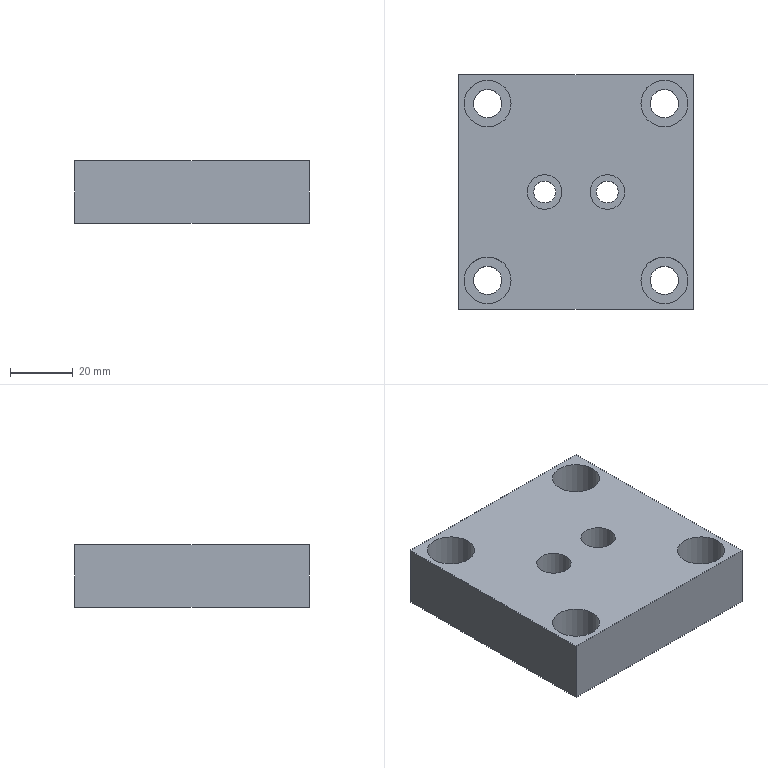Part | NX | features solid 2 | 1 solid | 24 faces | box 75 x 75 x 20 mm | volume 99312 mm3 | plane 12 | cylinder 12 | commonest cylinder face diameters 9 x4 15 x4 7 x2 11 x2
STEP:
#1=CARTESIAN_POINT('',(-127.5,292.5,330.));
#2=VERTEX_POINT('',#1);
#3=CARTESIAN_POINT('',(-127.5,292.5,350.));
#4=VERTEX_POINT('',#3);
#5=CARTESIAN_POINT('',(-127.5,292.5,350.));
#6=DIRECTION('',(0.,0.,-1.));
#7=VECTOR('',#6,1000.);
#8=LINE('',#5,#7);
#9=EDGE_CURVE('',#2,#4,#8,.F.);
#10=ORIENTED_EDGE('',*,*,#9,.T.);
#11=CARTESIAN_POINT('',(-52.5,292.5,350.));
#12=VERTEX_POINT('',#11);
#13=CARTESIAN_POINT('',(-205.,292.5,350.));
#14=DIRECTION('',(1.,0.,0.));
#15=VECTOR('',#14,1000.);
#16=LINE('',#13,#15);
#17=EDGE_CURVE('',#12,#4,#16,.F.);
#18=ORIENTED_EDGE('',*,*,#17,.F.);
#19=CARTESIAN_POINT('',(-52.5,292.5,330.));
#20=VERTEX_POINT('',#19);
#21=CARTESIAN_POINT('',(-52.5,292.5,350.));
#22=DIRECTION('',(0.,0.,1.));
#23=VECTOR('',#22,1000.);
#24=LINE('',#21,#23);
#25=EDGE_CURVE('',#20,#12,#24,.T.);
#26=ORIENTED_EDGE('',*,*,#25,.F.);
#27=CARTESIAN_POINT('',(-92.5,292.5,330.));
#28=DIRECTION('',(-1.,0.,0.));
#29=VECTOR('',#28,1000.);
#30=LINE('',#27,#29);
#31=EDGE_CURVE('',#20,#2,#30,.T.);
#32=ORIENTED_EDGE('',*,*,#31,.T.);
#33=EDGE_LOOP('',(#10,#18,#26,#32));
#34=FACE_BOUND('',#33,.T.);
#35=CARTESIAN_POINT('',(-62.5,292.5,350.));
#36=DIRECTION('',(0.,1.,0.));
#37=DIRECTION('',(-1.,0.,0.));
#38=AXIS2_PLACEMENT_3D('',#35,#36,#37);
#39=PLANE('',#38);
#40=ADVANCED_FACE('',(#34),#39,.T.);
#41=ORIENTED_EDGE('',*,*,#25,.T.);
#42=CARTESIAN_POINT('',(-52.5,217.5,350.));
#43=VERTEX_POINT('',#42);
#44=CARTESIAN_POINT('',(-52.5,50.,350.));
#45=DIRECTION('',(0.,-1.,0.));
#46=VECTOR('',#45,1000.);
#47=LINE('',#44,#46);
#48=EDGE_CURVE('',#43,#12,#47,.F.);
#49=ORIENTED_EDGE('',*,*,#48,.F.);
#50=CARTESIAN_POINT('',(-52.5,217.5,330.));
#51=VERTEX_POINT('',#50);
#52=CARTESIAN_POINT('',(-52.5,217.5,350.));
#53=DIRECTION('',(0.,0.,-1.));
#54=VECTOR('',#53,1000.);
#55=LINE('',#52,#54);
#56=EDGE_CURVE('',#51,#43,#55,.F.);
#57=ORIENTED_EDGE('',*,*,#56,.F.);
#58=CARTESIAN_POINT('',(-52.5,222.5,330.));
#59=DIRECTION('',(0.,1.,0.));
#60=VECTOR('',#59,1000.);
#61=LINE('',#58,#60);
#62=EDGE_CURVE('',#51,#20,#61,.T.);
#63=ORIENTED_EDGE('',*,*,#62,.T.);
#64=EDGE_LOOP('',(#41,#49,#57,#63));
#65=FACE_BOUND('',#64,.T.);
#66=CARTESIAN_POINT('',(-52.5,227.5,350.));
#67=DIRECTION('',(1.,0.,0.));
#68=DIRECTION('',(0.,0.,-1.));
#69=AXIS2_PLACEMENT_3D('',#66,#67,#68);
#70=PLANE('',#69);
#71=ADVANCED_FACE('',(#65),#70,.T.);
#72=ORIENTED_EDGE('',*,*,#56,.T.);
#73=CARTESIAN_POINT('',(-127.5,217.5,350.));
#74=VERTEX_POINT('',#73);
#75=CARTESIAN_POINT('',(-205.,217.5,350.));
#76=DIRECTION('',(-1.,0.,0.));
#77=VECTOR('',#76,1000.);
#78=LINE('',#75,#77);
#79=EDGE_CURVE('',#43,#74,#78,.T.);
#80=ORIENTED_EDGE('',*,*,#79,.T.);
#81=CARTESIAN_POINT('',(-127.5,217.5,330.));
#82=VERTEX_POINT('',#81);
#83=CARTESIAN_POINT('',(-127.5,217.5,350.));
#84=DIRECTION('',(0.,0.,1.));
#85=VECTOR('',#84,1000.);
#86=LINE('',#83,#85);
#87=EDGE_CURVE('',#82,#74,#86,.T.);
#88=ORIENTED_EDGE('',*,*,#87,.F.);
#89=CARTESIAN_POINT('',(-92.5,217.5,330.));
#90=DIRECTION('',(1.,0.,0.));
#91=VECTOR('',#90,1000.);
#92=LINE('',#89,#91);
#93=EDGE_CURVE('',#51,#82,#92,.F.);
#94=ORIENTED_EDGE('',*,*,#93,.F.);
#95=EDGE_LOOP('',(#72,#80,#88,#94));
#96=FACE_BOUND('',#95,.T.);
#97=CARTESIAN_POINT('',(-117.5,217.5,350.));
#98=DIRECTION('',(0.,-1.,0.));
#99=DIRECTION('',(0.,0.,-1.));
#100=AXIS2_PLACEMENT_3D('',#97,#98,#99);
#101=PLANE('',#100);
#102=ADVANCED_FACE('',(#96),#101,.T.);
#103=CARTESIAN_POINT('',(-127.5,50.,350.));
#104=DIRECTION('',(0.,1.,0.));
#105=VECTOR('',#104,1000.);
#106=LINE('',#103,#105);
#107=EDGE_CURVE('',#74,#4,#106,.T.);
#108=ORIENTED_EDGE('',*,*,#107,.T.);
#109=ORIENTED_EDGE('',*,*,#9,.F.);
#110=CARTESIAN_POINT('',(-127.5,222.5,330.));
#111=DIRECTION('',(0.,-1.,0.));
#112=VECTOR('',#111,1000.);
#113=LINE('',#110,#112);
#114=EDGE_CURVE('',#82,#2,#113,.F.);
#115=ORIENTED_EDGE('',*,*,#114,.F.);
#116=ORIENTED_EDGE('',*,*,#87,.T.);
#117=EDGE_LOOP('',(#108,#109,#115,#116));
#118=FACE_BOUND('',#117,.T.);
#119=CARTESIAN_POINT('',(-127.5,252.5,350.));
#120=DIRECTION('',(-1.,0.,0.));
#121=DIRECTION('',(0.,1.,0.));
#122=AXIS2_PLACEMENT_3D('',#119,#120,#121);
#123=PLANE('',#122);
#124=ADVANCED_FACE('',(#118),#123,.T.);
#125=CARTESIAN_POINT('',(-83.5,255.,330.));
#126=VERTEX_POINT('',#125);
#127=CARTESIAN_POINT('',(-80.,255.,330.));
#128=DIRECTION('',(0.,0.,-1.));
#129=DIRECTION('',(-1.,0.,0.));
#130=AXIS2_PLACEMENT_3D('',#127,#128,#129);
#131=CIRCLE('',#130,3.5);
#132=EDGE_CURVE('',#126,#126,#131,.T.);
#133=ORIENTED_EDGE('',*,*,#132,.F.);
#134=EDGE_LOOP('',(#133));
#135=FACE_BOUND('',#134,.T.);
#136=CARTESIAN_POINT('',(-103.5,255.,330.));
#137=VERTEX_POINT('',#136);
#138=CARTESIAN_POINT('',(-100.,255.,330.));
#139=DIRECTION('',(0.,0.,-1.));
#140=DIRECTION('',(-1.,0.,0.));
#141=AXIS2_PLACEMENT_3D('',#138,#139,#140);
#142=CIRCLE('',#141,3.5);
#143=EDGE_CURVE('',#137,#137,#142,.T.);
#144=ORIENTED_EDGE('',*,*,#143,.F.);
#145=EDGE_LOOP('',(#144));
#146=FACE_BOUND('',#145,.T.);
#147=CARTESIAN_POINT('',(-66.25,226.75,330.));
#148=VERTEX_POINT('',#147);
#149=CARTESIAN_POINT('',(-61.75,226.75,330.));
#150=DIRECTION('',(0.,0.,-1.));
#151=DIRECTION('',(-1.,0.,0.));
#152=AXIS2_PLACEMENT_3D('',#149,#150,#151);
#153=CIRCLE('',#152,4.5);
#154=EDGE_CURVE('',#148,#148,#153,.T.);
#155=ORIENTED_EDGE('',*,*,#154,.F.);
#156=EDGE_LOOP('',(#155));
#157=FACE_BOUND('',#156,.T.);
#158=CARTESIAN_POINT('',(-122.75,226.75,330.));
#159=VERTEX_POINT('',#158);
#160=CARTESIAN_POINT('',(-118.25,226.75,330.));
#161=DIRECTION('',(0.,0.,-1.));
#162=DIRECTION('',(-1.,0.,0.));
#163=AXIS2_PLACEMENT_3D('',#160,#161,#162);
#164=CIRCLE('',#163,4.5);
#165=EDGE_CURVE('',#159,#159,#164,.T.);
#166=ORIENTED_EDGE('',*,*,#165,.F.);
#167=EDGE_LOOP('',(#166));
#168=FACE_BOUND('',#167,.T.);
#169=CARTESIAN_POINT('',(-66.25,283.25,330.));
#170=VERTEX_POINT('',#169);
#171=CARTESIAN_POINT('',(-61.75,283.25,330.));
#172=DIRECTION('',(0.,0.,-1.));
#173=DIRECTION('',(-1.,0.,0.));
#174=AXIS2_PLACEMENT_3D('',#171,#172,#173);
#175=CIRCLE('',#174,4.5);
#176=EDGE_CURVE('',#170,#170,#175,.T.);
#177=ORIENTED_EDGE('',*,*,#176,.F.);
#178=EDGE_LOOP('',(#177));
#179=FACE_BOUND('',#178,.T.);
#180=CARTESIAN_POINT('',(-122.75,283.25,330.));
#181=VERTEX_POINT('',#180);
#182=CARTESIAN_POINT('',(-118.25,283.25,330.));
#183=DIRECTION('',(0.,0.,-1.));
#184=DIRECTION('',(-1.,0.,0.));
#185=AXIS2_PLACEMENT_3D('',#182,#183,#184);
#186=CIRCLE('',#185,4.5);
#187=EDGE_CURVE('',#181,#181,#186,.T.);
#188=ORIENTED_EDGE('',*,*,#187,.F.);
#189=EDGE_LOOP('',(#188));
#190=FACE_BOUND('',#189,.T.);
#191=ORIENTED_EDGE('',*,*,#31,.F.);
#192=ORIENTED_EDGE('',*,*,#62,.F.);
#193=ORIENTED_EDGE('',*,*,#93,.T.);
#194=ORIENTED_EDGE('',*,*,#114,.T.);
#195=EDGE_LOOP('',(#191,#192,#193,#194));
#196=FACE_BOUND('',#195,.T.);
#197=CARTESIAN_POINT('',(-92.5,222.5,330.));
#198=DIRECTION('',(0.,0.,-1.));
#199=DIRECTION('',(0.,1.,0.));
#200=AXIS2_PLACEMENT_3D('',#197,#198,#199);
#201=PLANE('',#200);
#202=ADVANCED_FACE('',(#135,#146,#157,#168,#179,#190,#196),#201,.T.);
#203=CARTESIAN_POINT('',(-85.5,255.,350.));
#204=VERTEX_POINT('',#203);
#205=CARTESIAN_POINT('',(-80.,255.,350.));
#206=DIRECTION('',(0.,0.,-1.));
#207=DIRECTION('',(-1.,0.,0.));
#208=AXIS2_PLACEMENT_3D('',#205,#206,#207);
#209=CIRCLE('',#208,5.5);
#210=EDGE_CURVE('',#204,#204,#209,.T.);
#211=ORIENTED_EDGE('',*,*,#210,.T.);
#212=EDGE_LOOP('',(#211));
#213=FACE_BOUND('',#212,.T.);
#214=CARTESIAN_POINT('',(-105.5,255.,350.));
#215=VERTEX_POINT('',#214);
#216=CARTESIAN_POINT('',(-100.,255.,350.));
#217=DIRECTION('',(0.,0.,-1.));
#218=DIRECTION('',(-1.,0.,0.));
#219=AXIS2_PLACEMENT_3D('',#216,#217,#218);
#220=CIRCLE('',#219,5.5);
#221=EDGE_CURVE('',#215,#215,#220,.T.);
#222=ORIENTED_EDGE('',*,*,#221,.T.);
#223=EDGE_LOOP('',(#222));
#224=FACE_BOUND('',#223,.T.);
#225=CARTESIAN_POINT('',(-69.25,226.75,350.));
#226=VERTEX_POINT('',#225);
#227=CARTESIAN_POINT('',(-61.75,226.75,350.));
#228=DIRECTION('',(0.,0.,-1.));
#229=DIRECTION('',(-1.,0.,0.));
#230=AXIS2_PLACEMENT_3D('',#227,#228,#229);
#231=CIRCLE('',#230,7.5);
#232=EDGE_CURVE('',#226,#226,#231,.T.);
#233=ORIENTED_EDGE('',*,*,#232,.T.);
#234=EDGE_LOOP('',(#233));
#235=FACE_BOUND('',#234,.T.);
#236=CARTESIAN_POINT('',(-125.75,226.75,350.));
#237=VERTEX_POINT('',#236);
#238=CARTESIAN_POINT('',(-118.25,226.75,350.));
#239=DIRECTION('',(0.,0.,-1.));
#240=DIRECTION('',(-1.,0.,0.));
#241=AXIS2_PLACEMENT_3D('',#238,#239,#240);
#242=CIRCLE('',#241,7.5);
#243=EDGE_CURVE('',#237,#237,#242,.T.);
#244=ORIENTED_EDGE('',*,*,#243,.T.);
#245=EDGE_LOOP('',(#244));
#246=FACE_BOUND('',#245,.T.);
#247=CARTESIAN_POINT('',(-69.25,283.25,350.));
#248=VERTEX_POINT('',#247);
#249=CARTESIAN_POINT('',(-61.75,283.25,350.));
#250=DIRECTION('',(0.,0.,-1.));
#251=DIRECTION('',(-1.,0.,0.));
#252=AXIS2_PLACEMENT_3D('',#249,#250,#251);
#253=CIRCLE('',#252,7.5);
#254=EDGE_CURVE('',#248,#248,#253,.T.);
#255=ORIENTED_EDGE('',*,*,#254,.T.);
#256=EDGE_LOOP('',(#255));
#257=FACE_BOUND('',#256,.T.);
#258=CARTESIAN_POINT('',(-125.75,283.25,350.));
#259=VERTEX_POINT('',#258);
#260=CARTESIAN_POINT('',(-118.25,283.25,350.));
#261=DIRECTION('',(0.,0.,-1.));
#262=DIRECTION('',(-1.,0.,0.));
#263=AXIS2_PLACEMENT_3D('',#260,#261,#262);
#264=CIRCLE('',#263,7.5);
#265=EDGE_CURVE('',#259,#259,#264,.T.);
#266=ORIENTED_EDGE('',*,*,#265,.T.);
#267=EDGE_LOOP('',(#266));
#268=FACE_BOUND('',#267,.T.);
#269=ORIENTED_EDGE('',*,*,#48,.T.);
#270=ORIENTED_EDGE('',*,*,#17,.T.);
#271=ORIENTED_EDGE('',*,*,#107,.F.);
#272=ORIENTED_EDGE('',*,*,#79,.F.);
#273=EDGE_LOOP('',(#269,#270,#271,#272));
#274=FACE_BOUND('',#273,.T.);
#275=CARTESIAN_POINT('',(-205.,50.,350.));
#276=DIRECTION('',(0.,0.,1.));
#277=DIRECTION('',(1.,0.,0.));
#278=AXIS2_PLACEMENT_3D('',#275,#276,#277);
#279=PLANE('',#278);
#280=ADVANCED_FACE('',(#213,#224,#235,#246,#257,#268,#274),#279,.T.);
#281=ORIENTED_EDGE('',*,*,#187,.T.);
#282=EDGE_LOOP('',(#281));
#283=FACE_BOUND('',#282,.T.);
#284=CARTESIAN_POINT('',(-122.75,283.25,338.));
#285=VERTEX_POINT('',#284);
#286=CARTESIAN_POINT('',(-118.25,283.25,338.));
#287=DIRECTION('',(0.,0.,-1.));
#288=DIRECTION('',(-1.,0.,0.));
#289=AXIS2_PLACEMENT_3D('',#286,#287,#288);
#290=CIRCLE('',#289,4.5);
#291=EDGE_CURVE('',#285,#285,#290,.T.);
#292=ORIENTED_EDGE('',*,*,#291,.F.);
#293=EDGE_LOOP('',(#292));
#294=FACE_BOUND('',#293,.T.);
#295=CARTESIAN_POINT('',(-118.25,283.25,300.));
#296=DIRECTION('',(0.,0.,-1.));
#297=DIRECTION('',(-1.,0.,0.));
#298=AXIS2_PLACEMENT_3D('',#295,#296,#297);
#299=CYLINDRICAL_SURFACE('',#298,4.5);
#300=ADVANCED_FACE('',(#283,#294),#299,.F.);
#301=ORIENTED_EDGE('',*,*,#291,.T.);
#302=EDGE_LOOP('',(#301));
#303=FACE_BOUND('',#302,.T.);
#304=CARTESIAN_POINT('',(-125.75,283.25,338.));
#305=VERTEX_POINT('',#304);
#306=CARTESIAN_POINT('',(-118.25,283.25,338.));
#307=DIRECTION('',(0.,0.,-1.));
#308=DIRECTION('',(-1.,0.,0.));
#309=AXIS2_PLACEMENT_3D('',#306,#307,#308);
#310=CIRCLE('',#309,7.5);
#311=EDGE_CURVE('',#305,#305,#310,.T.);
#312=ORIENTED_EDGE('',*,*,#311,.F.);
#313=EDGE_LOOP('',(#312));
#314=FACE_BOUND('',#313,.T.);
#315=CARTESIAN_POINT('',(-107.5,272.5,338.));
#316=DIRECTION('',(0.,0.,-1.));
#317=DIRECTION('',(-1.,0.,0.));
#318=AXIS2_PLACEMENT_3D('',#315,#316,#317);
#319=PLANE('',#318);
#320=ADVANCED_FACE('',(#303,#314),#319,.F.);
#321=ORIENTED_EDGE('',*,*,#311,.T.);
#322=EDGE_LOOP('',(#321));
#323=FACE_BOUND('',#322,.T.);
#324=ORIENTED_EDGE('',*,*,#265,.F.);
#325=EDGE_LOOP('',(#324));
#326=FACE_BOUND('',#325,.T.);
#327=CARTESIAN_POINT('',(-118.25,283.25,350.));
#328=DIRECTION('',(0.,0.,-1.));
#329=DIRECTION('',(-1.,0.,0.));
#330=AXIS2_PLACEMENT_3D('',#327,#328,#329);
#331=CYLINDRICAL_SURFACE('',#330,7.5);
#332=ADVANCED_FACE('',(#323,#326),#331,.F.);
#333=ORIENTED_EDGE('',*,*,#176,.T.);
#334=EDGE_LOOP('',(#333));
#335=FACE_BOUND('',#334,.T.);
#336=CARTESIAN_POINT('',(-66.25,283.25,338.));
#337=VERTEX_POINT('',#336);
#338=CARTESIAN_POINT('',(-61.75,283.25,338.));
#339=DIRECTION('',(0.,0.,-1.));
#340=DIRECTION('',(-1.,0.,0.));
#341=AXIS2_PLACEMENT_3D('',#338,#339,#340);
#342=CIRCLE('',#341,4.5);
#343=EDGE_CURVE('',#337,#337,#342,.T.);
#344=ORIENTED_EDGE('',*,*,#343,.F.);
#345=EDGE_LOOP('',(#344));
#346=FACE_BOUND('',#345,.T.);
#347=CARTESIAN_POINT('',(-61.75,283.25,300.));
#348=DIRECTION('',(0.,0.,-1.));
#349=DIRECTION('',(-1.,0.,0.));
#350=AXIS2_PLACEMENT_3D('',#347,#348,#349);
#351=CYLINDRICAL_SURFACE('',#350,4.5);
#352=ADVANCED_FACE('',(#335,#346),#351,.F.);
#353=ORIENTED_EDGE('',*,*,#343,.T.);
#354=EDGE_LOOP('',(#353));
#355=FACE_BOUND('',#354,.T.);
#356=CARTESIAN_POINT('',(-69.25,283.25,338.));
#357=VERTEX_POINT('',#356);
#358=CARTESIAN_POINT('',(-61.75,283.25,338.));
#359=DIRECTION('',(0.,0.,-1.));
#360=DIRECTION('',(-1.,0.,0.));
#361=AXIS2_PLACEMENT_3D('',#358,#359,#360);
#362=CIRCLE('',#361,7.5);
#363=EDGE_CURVE('',#357,#357,#362,.T.);
#364=ORIENTED_EDGE('',*,*,#363,.F.);
#365=EDGE_LOOP('',(#364));
#366=FACE_BOUND('',#365,.T.);
#367=CARTESIAN_POINT('',(-72.5,272.5,338.));
#368=DIRECTION('',(0.,0.,-1.));
#369=DIRECTION('',(-1.,0.,0.));
#370=AXIS2_PLACEMENT_3D('',#367,#368,#369);
#371=PLANE('',#370);
#372=ADVANCED_FACE('',(#355,#366),#371,.F.);
#373=ORIENTED_EDGE('',*,*,#363,.T.);
#374=EDGE_LOOP('',(#373));
#375=FACE_BOUND('',#374,.T.);
#376=ORIENTED_EDGE('',*,*,#254,.F.);
#377=EDGE_LOOP('',(#376));
#378=FACE_BOUND('',#377,.T.);
#379=CARTESIAN_POINT('',(-61.75,283.25,350.));
#380=DIRECTION('',(0.,0.,-1.));
#381=DIRECTION('',(-1.,0.,0.));
#382=AXIS2_PLACEMENT_3D('',#379,#380,#381);
#383=CYLINDRICAL_SURFACE('',#382,7.5);
#384=ADVANCED_FACE('',(#375,#378),#383,.F.);
#385=ORIENTED_EDGE('',*,*,#165,.T.);
#386=EDGE_LOOP('',(#385));
#387=FACE_BOUND('',#386,.T.);
#388=CARTESIAN_POINT('',(-122.75,226.75,338.));
#389=VERTEX_POINT('',#388);
#390=CARTESIAN_POINT('',(-118.25,226.75,338.));
#391=DIRECTION('',(0.,0.,-1.));
#392=DIRECTION('',(-1.,0.,0.));
#393=AXIS2_PLACEMENT_3D('',#390,#391,#392);
#394=CIRCLE('',#393,4.5);
#395=EDGE_CURVE('',#389,#389,#394,.T.);
#396=ORIENTED_EDGE('',*,*,#395,.F.);
#397=EDGE_LOOP('',(#396));
#398=FACE_BOUND('',#397,.T.);
#399=CARTESIAN_POINT('',(-118.25,226.75,300.));
#400=DIRECTION('',(0.,0.,-1.));
#401=DIRECTION('',(-1.,0.,0.));
#402=AXIS2_PLACEMENT_3D('',#399,#400,#401);
#403=CYLINDRICAL_SURFACE('',#402,4.5);
#404=ADVANCED_FACE('',(#387,#398),#403,.F.);
#405=ORIENTED_EDGE('',*,*,#395,.T.);
#406=EDGE_LOOP('',(#405));
#407=FACE_BOUND('',#406,.T.);
#408=CARTESIAN_POINT('',(-125.75,226.75,338.));
#409=VERTEX_POINT('',#408);
#410=CARTESIAN_POINT('',(-118.25,226.75,338.));
#411=DIRECTION('',(0.,0.,-1.));
#412=DIRECTION('',(-1.,0.,0.));
#413=AXIS2_PLACEMENT_3D('',#410,#411,#412);
#414=CIRCLE('',#413,7.5);
#415=EDGE_CURVE('',#409,#409,#414,.T.);
#416=ORIENTED_EDGE('',*,*,#415,.F.);
#417=EDGE_LOOP('',(#416));
#418=FACE_BOUND('',#417,.T.);
#419=CARTESIAN_POINT('',(-107.5,237.5,338.));
#420=DIRECTION('',(0.,0.,-1.));
#421=DIRECTION('',(-1.,0.,0.));
#422=AXIS2_PLACEMENT_3D('',#419,#420,#421);
#423=PLANE('',#422);
#424=ADVANCED_FACE('',(#407,#418),#423,.F.);
#425=ORIENTED_EDGE('',*,*,#415,.T.);
#426=EDGE_LOOP('',(#425));
#427=FACE_BOUND('',#426,.T.);
#428=ORIENTED_EDGE('',*,*,#243,.F.);
#429=EDGE_LOOP('',(#428));
#430=FACE_BOUND('',#429,.T.);
#431=CARTESIAN_POINT('',(-118.25,226.75,350.));
#432=DIRECTION('',(0.,0.,-1.));
#433=DIRECTION('',(-1.,0.,0.));
#434=AXIS2_PLACEMENT_3D('',#431,#432,#433);
#435=CYLINDRICAL_SURFACE('',#434,7.5);
#436=ADVANCED_FACE('',(#427,#430),#435,.F.);
#437=ORIENTED_EDGE('',*,*,#154,.T.);
#438=EDGE_LOOP('',(#437));
#439=FACE_BOUND('',#438,.T.);
#440=CARTESIAN_POINT('',(-66.25,226.75,338.));
#441=VERTEX_POINT('',#440);
#442=CARTESIAN_POINT('',(-61.75,226.75,338.));
#443=DIRECTION('',(0.,0.,-1.));
#444=DIRECTION('',(-1.,0.,0.));
#445=AXIS2_PLACEMENT_3D('',#442,#443,#444);
#446=CIRCLE('',#445,4.5);
#447=EDGE_CURVE('',#441,#441,#446,.T.);
#448=ORIENTED_EDGE('',*,*,#447,.F.);
#449=EDGE_LOOP('',(#448));
#450=FACE_BOUND('',#449,.T.);
#451=CARTESIAN_POINT('',(-61.75,226.75,300.));
#452=DIRECTION('',(0.,0.,-1.));
#453=DIRECTION('',(-1.,0.,0.));
#454=AXIS2_PLACEMENT_3D('',#451,#452,#453);
#455=CYLINDRICAL_SURFACE('',#454,4.5);
#456=ADVANCED_FACE('',(#439,#450),#455,.F.);
#457=ORIENTED_EDGE('',*,*,#447,.T.);
#458=EDGE_LOOP('',(#457));
#459=FACE_BOUND('',#458,.T.);
#460=CARTESIAN_POINT('',(-69.25,226.75,338.));
#461=VERTEX_POINT('',#460);
#462=CARTESIAN_POINT('',(-61.75,226.75,338.));
#463=DIRECTION('',(0.,0.,-1.));
#464=DIRECTION('',(-1.,0.,0.));
#465=AXIS2_PLACEMENT_3D('',#462,#463,#464);
#466=CIRCLE('',#465,7.5);
#467=EDGE_CURVE('',#461,#461,#466,.T.);
#468=ORIENTED_EDGE('',*,*,#467,.F.);
#469=EDGE_LOOP('',(#468));
#470=FACE_BOUND('',#469,.T.);
#471=CARTESIAN_POINT('',(-72.5,237.5,338.));
#472=DIRECTION('',(0.,0.,-1.));
#473=DIRECTION('',(-1.,0.,0.));
#474=AXIS2_PLACEMENT_3D('',#471,#472,#473);
#475=PLANE('',#474);
#476=ADVANCED_FACE('',(#459,#470),#475,.F.);
#477=ORIENTED_EDGE('',*,*,#467,.T.);
#478=EDGE_LOOP('',(#477));
#479=FACE_BOUND('',#478,.T.);
#480=ORIENTED_EDGE('',*,*,#232,.F.);
#481=EDGE_LOOP('',(#480));
#482=FACE_BOUND('',#481,.T.);
#483=CARTESIAN_POINT('',(-61.75,226.75,350.));
#484=DIRECTION('',(0.,0.,-1.));
#485=DIRECTION('',(-1.,0.,0.));
#486=AXIS2_PLACEMENT_3D('',#483,#484,#485);
#487=CYLINDRICAL_SURFACE('',#486,7.5);
#488=ADVANCED_FACE('',(#479,#482),#487,.F.);
#489=ORIENTED_EDGE('',*,*,#143,.T.);
#490=EDGE_LOOP('',(#489));
#491=FACE_BOUND('',#490,.T.);
#492=CARTESIAN_POINT('',(-103.5,255.,340.));
#493=VERTEX_POINT('',#492);
#494=CARTESIAN_POINT('',(-100.,255.,340.));
#495=DIRECTION('',(0.,0.,-1.));
#496=DIRECTION('',(-1.,0.,0.));
#497=AXIS2_PLACEMENT_3D('',#494,#495,#496);
#498=CIRCLE('',#497,3.5);
#499=EDGE_CURVE('',#493,#493,#498,.T.);
#500=ORIENTED_EDGE('',*,*,#499,.F.);
#501=EDGE_LOOP('',(#500));
#502=FACE_BOUND('',#501,.T.);
#503=CARTESIAN_POINT('',(-100.,255.,300.));
#504=DIRECTION('',(0.,0.,-1.));
#505=DIRECTION('',(-1.,0.,0.));
#506=AXIS2_PLACEMENT_3D('',#503,#504,#505);
#507=CYLINDRICAL_SURFACE('',#506,3.5);
#508=ADVANCED_FACE('',(#491,#502),#507,.F.);
#509=ORIENTED_EDGE('',*,*,#499,.T.);
#510=EDGE_LOOP('',(#509));
#511=FACE_BOUND('',#510,.T.);
#512=CARTESIAN_POINT('',(-105.5,255.,340.));
#513=VERTEX_POINT('',#512);
#514=CARTESIAN_POINT('',(-100.,255.,340.));
#515=DIRECTION('',(0.,0.,-1.));
#516=DIRECTION('',(-1.,0.,0.));
#517=AXIS2_PLACEMENT_3D('',#514,#515,#516);
#518=CIRCLE('',#517,5.5);
#519=EDGE_CURVE('',#513,#513,#518,.T.);
#520=ORIENTED_EDGE('',*,*,#519,.F.);
#521=EDGE_LOOP('',(#520));
#522=FACE_BOUND('',#521,.T.);
#523=CARTESIAN_POINT('',(-90.,255.,340.));
#524=DIRECTION('',(0.,0.,-1.));
#525=DIRECTION('',(-1.,0.,0.));
#526=AXIS2_PLACEMENT_3D('',#523,#524,#525);
#527=PLANE('',#526);
#528=ADVANCED_FACE('',(#511,#522),#527,.F.);
#529=ORIENTED_EDGE('',*,*,#519,.T.);
#530=EDGE_LOOP('',(#529));
#531=FACE_BOUND('',#530,.T.);
#532=ORIENTED_EDGE('',*,*,#221,.F.);
#533=EDGE_LOOP('',(#532));
#534=FACE_BOUND('',#533,.T.);
#535=CARTESIAN_POINT('',(-100.,255.,350.));
#536=DIRECTION('',(0.,0.,-1.));
#537=DIRECTION('',(-1.,0.,0.));
#538=AXIS2_PLACEMENT_3D('',#535,#536,#537);
#539=CYLINDRICAL_SURFACE('',#538,5.5);
#540=ADVANCED_FACE('',(#531,#534),#539,.F.);
#541=ORIENTED_EDGE('',*,*,#132,.T.);
#542=EDGE_LOOP('',(#541));
#543=FACE_BOUND('',#542,.T.);
#544=CARTESIAN_POINT('',(-83.5,255.,340.));
#545=VERTEX_POINT('',#544);
#546=CARTESIAN_POINT('',(-80.,255.,340.));
#547=DIRECTION('',(0.,0.,-1.));
#548=DIRECTION('',(-1.,0.,0.));
#549=AXIS2_PLACEMENT_3D('',#546,#547,#548);
#550=CIRCLE('',#549,3.5);
#551=EDGE_CURVE('',#545,#545,#550,.T.);
#552=ORIENTED_EDGE('',*,*,#551,.F.);
#553=EDGE_LOOP('',(#552));
#554=FACE_BOUND('',#553,.T.);
#555=CARTESIAN_POINT('',(-80.,255.,300.));
#556=DIRECTION('',(0.,0.,-1.));
#557=DIRECTION('',(-1.,0.,0.));
#558=AXIS2_PLACEMENT_3D('',#555,#556,#557);
#559=CYLINDRICAL_SURFACE('',#558,3.5);
#560=ADVANCED_FACE('',(#543,#554),#559,.F.);
#561=ORIENTED_EDGE('',*,*,#551,.T.);
#562=EDGE_LOOP('',(#561));
#563=FACE_BOUND('',#562,.T.);
#564=CARTESIAN_POINT('',(-85.5,255.,340.));
#565=VERTEX_POINT('',#564);
#566=CARTESIAN_POINT('',(-80.,255.,340.));
#567=DIRECTION('',(0.,0.,-1.));
#568=DIRECTION('',(-1.,0.,0.));
#569=AXIS2_PLACEMENT_3D('',#566,#567,#568);
#570=CIRCLE('',#569,5.5);
#571=EDGE_CURVE('',#565,#565,#570,.T.);
#572=ORIENTED_EDGE('',*,*,#571,.F.);
#573=EDGE_LOOP('',(#572));
#574=FACE_BOUND('',#573,.T.);
#575=CARTESIAN_POINT('',(-77.5,255.,340.));
#576=DIRECTION('',(0.,0.,-1.));
#577=DIRECTION('',(-1.,0.,0.));
#578=AXIS2_PLACEMENT_3D('',#575,#576,#577);
#579=PLANE('',#578);
#580=ADVANCED_FACE('',(#563,#574),#579,.F.);
#581=ORIENTED_EDGE('',*,*,#571,.T.);
#582=EDGE_LOOP('',(#581));
#583=FACE_BOUND('',#582,.T.);
#584=ORIENTED_EDGE('',*,*,#210,.F.);
#585=EDGE_LOOP('',(#584));
#586=FACE_BOUND('',#585,.T.);
#587=CARTESIAN_POINT('',(-80.,255.,350.));
#588=DIRECTION('',(0.,0.,-1.));
#589=DIRECTION('',(-1.,0.,0.));
#590=AXIS2_PLACEMENT_3D('',#587,#588,#589);
#591=CYLINDRICAL_SURFACE('',#590,5.5);
#592=ADVANCED_FACE('',(#583,#586),#591,.F.);
#593=CLOSED_SHELL('',(#40,#71,#102,#124,#202,#280,#300,#320,#332,#352,#372,#384,#404,#424,#436,#456,#476,#488,#508,#528,#540,#560,#580,#592));
#594=MANIFOLD_SOLID_BREP('',#593);
#595=(LENGTH_UNIT()NAMED_UNIT(*)SI_UNIT(.MILLI.,.METRE.));
#596=UNCERTAINTY_MEASURE_WITH_UNIT(LENGTH_MEASURE(0.00001),#595,'','');
#597=(NAMED_UNIT(*)PLANE_ANGLE_UNIT()SI_UNIT($,.RADIAN.));
#598=(NAMED_UNIT(*)SI_UNIT($,.STERADIAN.)SOLID_ANGLE_UNIT());
#599=(GEOMETRIC_REPRESENTATION_CONTEXT(3)GLOBAL_UNCERTAINTY_ASSIGNED_CONTEXT((#596))GLOBAL_UNIT_ASSIGNED_CONTEXT((#595,#597,#598))REPRESENTATION_CONTEXT('',''));
#600=ADVANCED_BREP_SHAPE_REPRESENTATION('',(#594),#599);